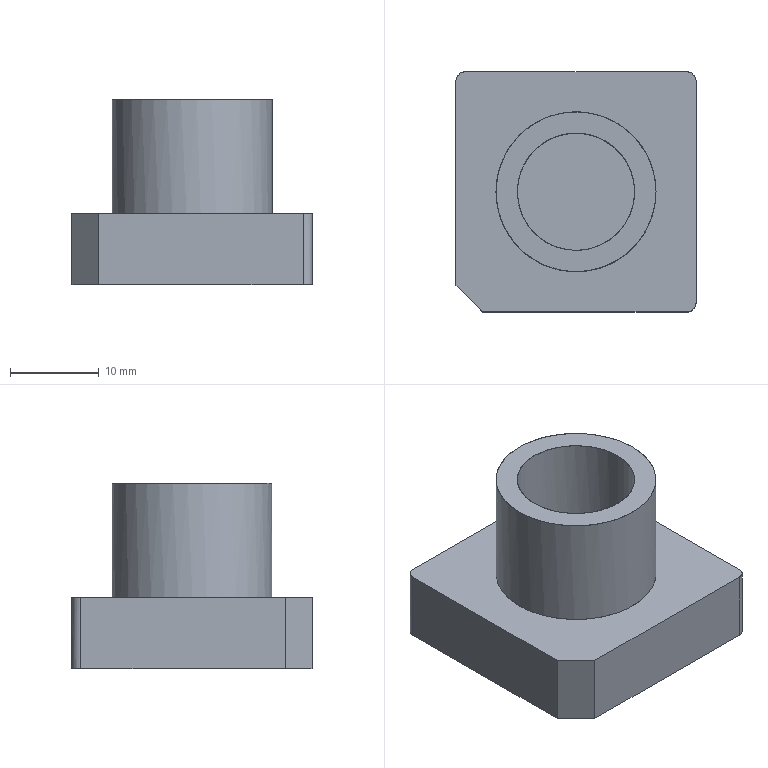NC program | PowerMill | posted with a generic post | part box 27 x 27 x 20.913 mm
Lines 4984 to 6006 of 92133:
N5081 M6
N5082 S18000 M03
N5083 G00 G90 X0.0 Y0.0
N5084 G43 Z9.8026 H2
N5085
N5086 G05 P10000 R4
N5087 X6.8917 Y9.7829
N5088 Z0.7935
N5089 G01 Z-0.4065 F3600.0
N5090 X6.8713 Y9.7747 F6000.0
N5091 G03 X6.762 Y9.5169 I0.0742 J-0.1836
N5092 G01 X7.2898 Y8.2119
N5093 X7.7468 Y7.8088
N5094 X8.2969 Y7.2124
N5095 X8.9814 Y6.3447
N5096 X9.6009 Y5.3686
N5097 X10.0822 Y4.3925
N5098 X10.451 Y3.4164
N5099 X10.7253 Y2.4403
N5100 X10.8209 Y1.9522
N5101 X10.9546 Y0.9761
N5102 X11.0 Y0.0
N5103 X10.9546 Y-0.9761
N5104 X10.8953 Y-1.4642
N5105 X10.7253 Y-2.4403
N5106 X10.451 Y-3.4164
N5107 X10.0822 Y-4.3925
N5108 X9.6009 Y-5.3686
N5109 X9.273 Y-5.9165
N5110 X8.6143 Y-6.8327
N5111 X7.8088 Y-7.7468
N5112 X7.2124 Y-8.2969
N5113 X6.3447 Y-8.9814
N5114 X5.3686 Y-9.6009
N5115 X4.3925 Y-10.0822
N5116 X3.4164 Y-10.4559
N5117 X2.3638 Y-10.7372
N5118 X1.9522 Y-10.8209
N5119 X0.9761 Y-10.9563
N5120 X0.0 Y-11.0
N5121 X-0.9761 Y-10.9546
N5122 X-1.9522 Y-10.8209
N5123 X-2.9283 Y-10.5992
N5124 X-3.9944 Y-10.2491
N5125 X-4.3925 Y-10.0822
N5126 X-5.3686 Y-9.6009
N5127 X-6.3447 Y-8.9814
N5128 X-7.222 Y-8.2969
N5129 X-7.7468 Y-7.8088
N5130 X-8.2041 Y-7.3208
N5131 X-8.6121 Y-6.8327
N5132 X-8.9814 Y-6.3447
N5133 X-9.6009 Y-5.3686
N5134 X-10.0822 Y-4.3925
N5135 X-10.451 Y-3.4164
N5136 X-10.5975 Y-2.9283
N5137 X-10.8241 Y-1.9522
N5138 X-10.9546 Y-0.9761
N5139 X-11.0 Y0.0
N5140 X-10.9546 Y0.9761
N5141 X-10.8241 Y1.9522
N5142 X-10.7198 Y2.4403
N5143 X-10.451 Y3.4164
N5144 X-10.0822 Y4.3925
N5145 X-9.6009 Y5.3686
N5146 X-9.3005 Y5.8566
N5147 X-8.7849 Y6.6104
N5148 X-8.2041 Y7.3208
N5149 X-7.8088 Y7.7468
N5150 X-7.222 Y8.2969
N5151 X-6.3447 Y8.9814
N5152 X-5.9008 Y9.273
N5153 X-5.0694 Y9.7611
N5154 X-3.9944 Y10.2491
N5155 X-2.9283 Y10.5992
N5156 X-1.9522 Y10.8209
N5157 X-0.9761 Y10.9546
N5158 X0.0 Y11.0
N5159 X0.9761 Y10.9563
N5160 X1.4642 Y10.8953
N5161 X2.3638 Y10.7372
N5162 X3.4164 Y10.4559
N5163 X4.3925 Y10.0822
N5164 X5.3686 Y9.6009
N5165 X6.3447 Y8.9814
N5166 X6.8327 Y8.6151
N5167 X7.2898 Y8.2119
N5168 X6.8917 Y9.7829 Z-0.606
N5169 X6.8713 Y9.7747
N5170 G03 X6.762 Y9.5169 I0.0742 J-0.1836
N5171 G01 X7.2898 Y8.2119
N5172 X7.7468 Y7.8088
N5173 X8.2969 Y7.2124
N5174 X8.9814 Y6.3447
N5175 X9.6009 Y5.3686
N5176 X10.0822 Y4.3925
N5177 X10.451 Y3.4164
N5178 X10.7253 Y2.4403
N5179 X10.8209 Y1.9522
N5180 X10.9546 Y0.9761
N5181 X11.0 Y0.0
N5182 X10.9546 Y-0.9761
N5183 X10.8953 Y-1.4642
N5184 X10.7253 Y-2.4403
N5185 X10.451 Y-3.4164
N5186 X10.0822 Y-4.3925
N5187 X9.6009 Y-5.3686
N5188 X9.273 Y-5.9165
N5189 X8.6143 Y-6.8327
N5190 X7.8088 Y-7.7468
N5191 X7.2124 Y-8.2969
N5192 X6.3447 Y-8.9814
N5193 X5.3686 Y-9.6009
N5194 X4.3925 Y-10.0822
N5195 X3.4164 Y-10.4559
N5196 X2.3638 Y-10.7372
N5197 X1.9522 Y-10.8209
N5198 X0.9761 Y-10.9563
N5199 X0.0 Y-11.0
N5200 X-0.9761 Y-10.9546
N5201 X-1.9522 Y-10.8209
N5202 X-2.9283 Y-10.5992
N5203 X-3.9944 Y-10.2491
N5204 X-4.3925 Y-10.0822
N5205 X-5.3686 Y-9.6009
N5206 X-6.3447 Y-8.9814
N5207 X-7.2221 Y-8.2969
N5208 X-7.7468 Y-7.8088
N5209 X-8.2041 Y-7.3208
N5210 X-8.6121 Y-6.8327
N5211 X-8.9814 Y-6.3447
N5212 X-9.6009 Y-5.3686
N5213 X-10.0822 Y-4.3925
N5214 X-10.451 Y-3.4164
N5215 X-10.5975 Y-2.9283
N5216 X-10.8241 Y-1.9522
N5217 X-10.9546 Y-0.9761
N5218 X-11.0 Y0.0
N5219 X-10.9546 Y0.9761
N5220 X-10.8241 Y1.9522
N5221 X-10.7198 Y2.4403
N5222 X-10.451 Y3.4164
N5223 X-10.0822 Y4.3925
N5224 X-9.6009 Y5.3686
N5225 X-9.3005 Y5.8566
N5226 X-8.7849 Y6.6104
N5227 X-8.2041 Y7.3208
N5228 X-7.8088 Y7.7468
N5229 X-7.2221 Y8.2969
N5230 X-6.3447 Y8.9814
N5231 X-5.9008 Y9.273
N5232 X-5.0694 Y9.7611
N5233 X-3.9944 Y10.2491
N5234 X-2.9283 Y10.5992
N5235 X-1.9522 Y10.8209
N5236 X-0.9761 Y10.9546
N5237 X0.0 Y11.0
N5238 X0.9761 Y10.9563
N5239 X1.4642 Y10.8953
N5240 X2.3638 Y10.7372
N5241 X3.4164 Y10.4559
N5242 X4.3925 Y10.0822
N5243 X5.3686 Y9.6009
N5244 X6.3447 Y8.9814
N5245 X6.8327 Y8.6151
N5246 X7.2898 Y8.2119
N5247 X6.8917 Y9.7829 Z-0.8056
N5248 X6.8713 Y9.7747
N5249 G03 X6.762 Y9.5169 I0.0742 J-0.1836
N5250 G01 X7.2898 Y8.2119
N5251 X7.7468 Y7.8088
N5252 X8.2969 Y7.2124
N5253 X8.9814 Y6.3447
N5254 X9.6009 Y5.3686
N5255 X10.0822 Y4.3925
N5256 X10.451 Y3.4164
N5257 X10.7253 Y2.4403
N5258 X10.8209 Y1.9522
N5259 X10.9546 Y0.9761
N5260 X11.0 Y0.0
N5261 X10.9546 Y-0.9761
N5262 X10.8953 Y-1.4642
N5263 X10.7253 Y-2.4403
N5264 X10.451 Y-3.4164
N5265 X10.0822 Y-4.3925
N5266 X9.6009 Y-5.3686
N5267 X9.273 Y-5.9165
N5268 X8.6143 Y-6.8327
N5269 X7.8088 Y-7.7468
N5270 X7.2124 Y-8.2969
N5271 X6.3447 Y-8.9814
N5272 X5.3686 Y-9.6009
N5273 X4.3925 Y-10.0822
N5274 X3.4164 Y-10.4559
N5275 X2.3638 Y-10.7372
N5276 X1.9522 Y-10.8209
N5277 X0.9761 Y-10.9563
N5278 X0.0 Y-11.0
N5279 X-0.9761 Y-10.9546
N5280 X-1.9522 Y-10.8209
N5281 X-2.9283 Y-10.5992
N5282 X-3.9944 Y-10.2491
N5283 X-4.3925 Y-10.0822
N5284 X-5.3686 Y-9.6009
N5285 X-6.3447 Y-8.9814
N5286 X-7.2221 Y-8.2969
N5287 X-7.7468 Y-7.8088
N5288 X-8.2041 Y-7.3208
N5289 X-8.6121 Y-6.8327
N5290 X-8.9814 Y-6.3447
N5291 X-9.6009 Y-5.3686
N5292 X-10.0822 Y-4.3925
N5293 X-10.451 Y-3.4164
N5294 X-10.5975 Y-2.9283
N5295 X-10.8241 Y-1.9522
N5296 X-10.9546 Y-0.9761
N5297 X-11.0 Y0.0
N5298 X-10.9546 Y0.9761
N5299 X-10.8241 Y1.9522
N5300 X-10.7198 Y2.4403
N5301 X-10.451 Y3.4164
N5302 X-10.0822 Y4.3925
N5303 X-9.6009 Y5.3686
N5304 X-9.3005 Y5.8566
N5305 X-8.7849 Y6.6104
N5306 X-8.2041 Y7.3208
N5307 X-7.8088 Y7.7468
N5308 X-7.2221 Y8.2969
N5309 X-6.3447 Y8.9814
N5310 X-5.9008 Y9.273
N5311 X-5.0694 Y9.7611
N5312 X-3.9944 Y10.2491
N5313 X-2.9283 Y10.5992
N5314 X-1.9522 Y10.8209
N5315 X-0.9761 Y10.9546
N5316 X0.0 Y11.0
N5317 X0.9761 Y10.9563
N5318 X1.4642 Y10.8953
N5319 X2.3638 Y10.7372
N5320 X3.4164 Y10.4559
N5321 X4.3925 Y10.0822
N5322 X5.3686 Y9.6009
N5323 X6.3447 Y8.9814
N5324 X6.8327 Y8.6151
N5325 X7.2898 Y8.2119
N5326 X6.8917 Y9.7829 Z-1.0051
N5327 X6.8713 Y9.7747
N5328 G03 X6.762 Y9.5169 I0.0742 J-0.1836
N5329 G01 X7.2898 Y8.2119
N5330 X7.7468 Y7.8088
N5331 X8.2969 Y7.2125
N5332 X8.9814 Y6.3447
N5333 X9.6009 Y5.3686
N5334 X10.0822 Y4.3925
N5335 X10.451 Y3.4164
N5336 X10.7253 Y2.4403
N5337 X10.8209 Y1.9522
N5338 X10.9546 Y0.9761
N5339 X11.0 Y0.0
N5340 X10.9546 Y-0.9761
N5341 X10.8953 Y-1.4642
N5342 X10.7253 Y-2.4403
N5343 X10.451 Y-3.4164
N5344 X10.0822 Y-4.3925
N5345 X9.6009 Y-5.3686
N5346 X9.273 Y-5.9165
N5347 X8.6143 Y-6.8327
N5348 X7.8088 Y-7.7468
N5349 X7.2125 Y-8.2969
N5350 X6.3447 Y-8.9814
N5351 X5.3686 Y-9.6009
N5352 X4.3925 Y-10.0822
N5353 X3.4164 Y-10.4559
N5354 X2.3638 Y-10.7372
N5355 X1.9522 Y-10.8209
N5356 X0.9761 Y-10.9563
N5357 X0.0 Y-11.0
N5358 X-0.9761 Y-10.9546
N5359 X-1.9522 Y-10.8209
N5360 X-2.9283 Y-10.5992
N5361 X-3.9944 Y-10.2491
N5362 X-4.3925 Y-10.0822
N5363 X-5.3686 Y-9.6009
N5364 X-6.3447 Y-8.9814
N5365 X-7.2221 Y-8.2969
N5366 X-7.7468 Y-7.8088
N5367 X-8.2041 Y-7.3208
N5368 X-8.6121 Y-6.8327
N5369 X-8.9814 Y-6.3447
N5370 X-9.6009 Y-5.3686
N5371 X-10.0822 Y-4.3925
N5372 X-10.451 Y-3.4164
N5373 X-10.5975 Y-2.9283
N5374 X-10.8241 Y-1.9522
N5375 X-10.9546 Y-0.9761
N5376 X-11.0 Y0.0
N5377 X-10.9546 Y0.9761
N5378 X-10.8241 Y1.9522
N5379 X-10.7198 Y2.4403
N5380 X-10.451 Y3.4164
N5381 X-10.0822 Y4.3925
N5382 X-9.6009 Y5.3686
N5383 X-9.3005 Y5.8566
N5384 X-8.7849 Y6.6104
N5385 X-8.2041 Y7.3208
N5386 X-7.8088 Y7.7468
N5387 X-7.2221 Y8.2969
N5388 X-6.3447 Y8.9814
N5389 X-5.9008 Y9.273
N5390 X-5.0694 Y9.7611
N5391 X-3.9944 Y10.2491
N5392 X-2.9283 Y10.5992
N5393 X-1.9522 Y10.8209
N5394 X-0.9761 Y10.9546
N5395 X0.0 Y11.0
N5396 X0.9761 Y10.9563
N5397 X1.4642 Y10.8953
N5398 X2.3638 Y10.7372
N5399 X3.4164 Y10.4559
N5400 X4.3925 Y10.0822
N5401 X5.3686 Y9.6009
N5402 X6.3447 Y8.9814
N5403 X6.8327 Y8.6151
N5404 X7.2898 Y8.2119
N5405 X6.8917 Y9.7829 Z-1.2046
N5406 X6.8713 Y9.7747
N5407 G03 X6.762 Y9.5169 I0.0742 J-0.1836
N5408 G01 X7.2898 Y8.212
N5409 X7.7468 Y7.8088
N5410 X8.2969 Y7.2125
N5411 X8.9814 Y6.3447
N5412 X9.6009 Y5.3686
N5413 X10.0822 Y4.3925
N5414 X10.451 Y3.4164
N5415 X10.7253 Y2.4403
N5416 X10.8209 Y1.9522
N5417 X10.9546 Y0.9761
N5418 X11.0 Y0.0
N5419 X10.9546 Y-0.9761
N5420 X10.8953 Y-1.4642
N5421 X10.7253 Y-2.4403
N5422 X10.451 Y-3.4164
N5423 X10.0822 Y-4.3925
N5424 X9.6009 Y-5.3686
N5425 X9.273 Y-5.9165
N5426 X8.6143 Y-6.8327
N5427 X7.8088 Y-7.7468
N5428 X7.2125 Y-8.2969
N5429 X6.3447 Y-8.9814
N5430 X5.3686 Y-9.6009
N5431 X4.3925 Y-10.0822
N5432 X3.4164 Y-10.4559
N5433 X2.3638 Y-10.7372
N5434 X1.9522 Y-10.8209
N5435 X0.9761 Y-10.9563
N5436 X0.0 Y-11.0
N5437 X-0.9761 Y-10.9546
N5438 X-1.9522 Y-10.8209
N5439 X-2.9283 Y-10.5992
N5440 X-3.9944 Y-10.2491
N5441 X-4.3925 Y-10.0822
N5442 X-5.3686 Y-9.6009
N5443 X-6.3447 Y-8.9814
N5444 X-7.2221 Y-8.2969
N5445 X-7.7468 Y-7.8088
N5446 X-8.2041 Y-7.3208
N5447 X-8.6121 Y-6.8327
N5448 X-8.9814 Y-6.3447
N5449 X-9.6009 Y-5.3686
N5450 X-10.0822 Y-4.3925
N5451 X-10.451 Y-3.4164
N5452 X-10.5975 Y-2.9283
N5453 X-10.8241 Y-1.9522
N5454 X-10.9546 Y-0.9761
N5455 X-11.0 Y0.0
N5456 X-10.9546 Y0.9761
N5457 X-10.8241 Y1.9522
N5458 X-10.7198 Y2.4403
N5459 X-10.451 Y3.4164
N5460 X-10.0822 Y4.3925
N5461 X-9.6009 Y5.3686
N5462 X-9.3005 Y5.8566
N5463 X-8.7849 Y6.6104
N5464 X-8.2041 Y7.3208
N5465 X-7.8088 Y7.7468
N5466 X-7.2221 Y8.2969
N5467 X-6.3447 Y8.9814
N5468 X-5.9008 Y9.273
N5469 X-5.0694 Y9.7611
N5470 X-3.9944 Y10.2491
N5471 X-2.9283 Y10.5992
N5472 X-1.9522 Y10.8209
N5473 X-0.9761 Y10.9546
N5474 X0.0 Y11.0
N5475 X0.9761 Y10.9563
N5476 X1.4642 Y10.8953
N5477 X2.3638 Y10.7372
N5478 X3.4164 Y10.4559
N5479 X4.3925 Y10.0822
N5480 X5.3686 Y9.6009
N5481 X6.3447 Y8.9814
N5482 X6.8327 Y8.6151
N5483 X7.2898 Y8.212
N5484 X6.8917 Y9.7829 Z-1.4041
N5485 X6.8713 Y9.7747
N5486 G03 X6.762 Y9.5169 I0.0742 J-0.1836
N5487 G01 X7.2898 Y8.212
N5488 X7.7468 Y7.8088
N5489 X8.2969 Y7.2125
N5490 X8.9814 Y6.3447
N5491 X9.6009 Y5.3686
N5492 X10.0822 Y4.3925
N5493 X10.451 Y3.4164
N5494 X10.7253 Y2.4403
N5495 X10.8209 Y1.9522
N5496 X10.9546 Y0.9761
N5497 X11.0 Y0.0
N5498 X10.9546 Y-0.9761
N5499 X10.8953 Y-1.4642
N5500 X10.7253 Y-2.4403
N5501 X10.451 Y-3.4164
N5502 X10.0822 Y-4.3925
N5503 X9.6009 Y-5.3686
N5504 X9.273 Y-5.9165
N5505 X8.6143 Y-6.8327
N5506 X7.8088 Y-7.7468
N5507 X7.2125 Y-8.2969
N5508 X6.3447 Y-8.9814
N5509 X5.3686 Y-9.6009
N5510 X4.3925 Y-10.0822
N5511 X3.4164 Y-10.4559
N5512 X2.3638 Y-10.7372
N5513 X1.9522 Y-10.8209
N5514 X0.9761 Y-10.9563
N5515 X0.0 Y-11.0
N5516 X-0.9761 Y-10.9546
N5517 X-1.9522 Y-10.8209
N5518 X-2.9283 Y-10.5992
N5519 X-3.9944 Y-10.2491
N5520 X-4.3925 Y-10.0822
N5521 X-5.3686 Y-9.6009
N5522 X-6.3447 Y-8.9814
N5523 X-7.2221 Y-8.2969
N5524 X-7.7468 Y-7.8088
N5525 X-8.2041 Y-7.3208
N5526 X-8.6121 Y-6.8327
N5527 X-8.9814 Y-6.3447
N5528 X-9.6009 Y-5.3686
N5529 X-10.0822 Y-4.3925
N5530 X-10.451 Y-3.4164
N5531 X-10.5975 Y-2.9283
N5532 X-10.8241 Y-1.9522
N5533 X-10.9546 Y-0.9761
N5534 X-11.0 Y0.0
N5535 X-10.9546 Y0.9761
N5536 X-10.8241 Y1.9522
N5537 X-10.7198 Y2.4403
N5538 X-10.451 Y3.4164
N5539 X-10.0822 Y4.3925
N5540 X-9.6009 Y5.3686
N5541 X-9.3005 Y5.8566
N5542 X-8.7849 Y6.6104
N5543 X-8.2041 Y7.3208
N5544 X-7.8088 Y7.7468
N5545 X-7.2221 Y8.2969
N5546 X-6.3447 Y8.9814
N5547 X-5.9008 Y9.273
N5548 X-5.0694 Y9.7611
N5549 X-3.9944 Y10.2491
N5550 X-2.9283 Y10.5992
N5551 X-1.9522 Y10.8209
N5552 X-0.9761 Y10.9546
N5553 X0.0 Y11.0
N5554 X0.9761 Y10.9563
N5555 X1.4642 Y10.8953
N5556 X2.3638 Y10.7372
N5557 X3.4164 Y10.4559
N5558 X4.3925 Y10.0822
N5559 X5.3686 Y9.6009
N5560 X6.3447 Y8.9814
N5561 X6.8327 Y8.6151
N5562 X7.2898 Y8.212
N5563 X6.8917 Y9.7829 Z-1.6037
N5564 X6.8713 Y9.7747
N5565 G03 X6.762 Y9.5169 I0.0742 J-0.1836
N5566 G01 X7.2898 Y8.212
N5567 X7.7468 Y7.8088
N5568 X8.2969 Y7.2125
N5569 X8.9814 Y6.3447
N5570 X9.6009 Y5.3686
N5571 X10.0822 Y4.3925
N5572 X10.451 Y3.4164
N5573 X10.7253 Y2.4403
N5574 X10.8209 Y1.9522
N5575 X10.9546 Y0.9761
N5576 X11.0 Y0.0
N5577 X10.9546 Y-0.9761
N5578 X10.8953 Y-1.4642
N5579 X10.7253 Y-2.4403
N5580 X10.451 Y-3.4164
N5581 X10.0822 Y-4.3925
N5582 X9.6009 Y-5.3686
N5583 X9.273 Y-5.9165
N5584 X8.6143 Y-6.8327
N5585 X7.8088 Y-7.7468
N5586 X7.2125 Y-8.2969
N5587 X6.3447 Y-8.9814
N5588 X5.3686 Y-9.6009
N5589 X4.3925 Y-10.0822
N5590 X3.4164 Y-10.4559
N5591 X2.3638 Y-10.7372
N5592 X1.9522 Y-10.8209
N5593 X0.9761 Y-10.9563
N5594 X0.0 Y-11.0
N5595 X-0.9761 Y-10.9546
N5596 X-1.9522 Y-10.8209
N5597 X-2.9283 Y-10.5992
N5598 X-3.9944 Y-10.2491
N5599 X-4.3925 Y-10.0822
N5600 X-5.3686 Y-9.6009
N5601 X-6.3447 Y-8.9814
N5602 X-7.2221 Y-8.2969
N5603 X-7.7468 Y-7.8088
N5604 X-8.2041 Y-7.3208
N5605 X-8.6121 Y-6.8327
N5606 X-8.9814 Y-6.3447
N5607 X-9.6009 Y-5.3686
N5608 X-10.0822 Y-4.3925
N5609 X-10.451 Y-3.4164
N5610 X-10.5975 Y-2.9283
N5611 X-10.8241 Y-1.9522
N5612 X-10.9546 Y-0.9761
N5613 X-11.0 Y0.0
N5614 X-10.9546 Y0.9761
N5615 X-10.8241 Y1.9522
N5616 X-10.7198 Y2.4403
N5617 X-10.451 Y3.4164
N5618 X-10.0822 Y4.3925
N5619 X-9.6009 Y5.3686
N5620 X-9.3005 Y5.8566
N5621 X-8.7849 Y6.6104
N5622 X-8.2041 Y7.3208
N5623 X-7.8088 Y7.7468
N5624 X-7.2221 Y8.2969
N5625 X-6.3447 Y8.9814
N5626 X-5.9008 Y9.273
N5627 X-5.0694 Y9.7611
N5628 X-3.9944 Y10.2491
N5629 X-2.9283 Y10.5992
N5630 X-1.9522 Y10.8209
N5631 X-0.9761 Y10.9546
N5632 X0.0 Y11.0
N5633 X0.9761 Y10.9563
N5634 X1.4642 Y10.8953
N5635 X2.3638 Y10.7372
N5636 X3.4164 Y10.4559
N5637 X4.3925 Y10.0822
N5638 X5.3686 Y9.6009
N5639 X6.3447 Y8.9814
N5640 X6.8327 Y8.6151
N5641 X7.2898 Y8.212
N5642 X6.8917 Y9.7829 Z-1.8032
N5643 X6.8713 Y9.7747
N5644 G03 X6.762 Y9.5169 I0.0742 J-0.1836
N5645 G01 X7.2898 Y8.212
N5646 X7.7468 Y7.8088
N5647 X8.2969 Y7.2125
N5648 X8.9814 Y6.3447
N5649 X9.6009 Y5.3686
N5650 X10.0822 Y4.3925
N5651 X10.451 Y3.4164
N5652 X10.7253 Y2.4403
N5653 X10.8209 Y1.9522
N5654 X10.9546 Y0.9761
N5655 X11.0 Y0.0
N5656 X10.9546 Y-0.9761
N5657 X10.8953 Y-1.4642
N5658 X10.7253 Y-2.4403
N5659 X10.451 Y-3.4164
N5660 X10.0822 Y-4.3925
N5661 X9.6009 Y-5.3686
N5662 X9.273 Y-5.9165
N5663 X8.6143 Y-6.8327
N5664 X7.8088 Y-7.7468
N5665 X7.2125 Y-8.2969
N5666 X6.3447 Y-8.9814
N5667 X5.3686 Y-9.6009
N5668 X4.3925 Y-10.0822
N5669 X3.4164 Y-10.4559
N5670 X2.3638 Y-10.7372
N5671 X1.9522 Y-10.8209
N5672 X0.9761 Y-10.9563
N5673 X0.0 Y-11.0
N5674 X-0.9761 Y-10.9546
N5675 X-1.9522 Y-10.8209
N5676 X-2.9283 Y-10.5992
N5677 X-3.9944 Y-10.2491
N5678 X-4.3925 Y-10.0822
N5679 X-5.3686 Y-9.6009
N5680 X-6.3447 Y-8.9814
N5681 X-7.2221 Y-8.2969
N5682 X-7.7468 Y-7.8088
N5683 X-8.2041 Y-7.3208
N5684 X-8.6121 Y-6.8327
N5685 X-8.9814 Y-6.3447
N5686 X-9.6009 Y-5.3686
N5687 X-10.0822 Y-4.3925
N5688 X-10.451 Y-3.4164
N5689 X-10.5975 Y-2.9283
N5690 X-10.8241 Y-1.9522
N5691 X-10.9546 Y-0.9761
N5692 X-11.0 Y0.0
N5693 X-10.9546 Y0.9761
N5694 X-10.8241 Y1.9522
N5695 X-10.7198 Y2.4403
N5696 X-10.451 Y3.4164
N5697 X-10.0822 Y4.3925
N5698 X-9.6009 Y5.3686
N5699 X-9.3005 Y5.8566
N5700 X-8.7849 Y6.6104
N5701 X-8.2041 Y7.3208
N5702 X-7.8088 Y7.7468
N5703 X-7.2221 Y8.2969
N5704 X-6.3447 Y8.9814
N5705 X-5.9008 Y9.273
N5706 X-5.0694 Y9.7611
N5707 X-3.9944 Y10.2491
N5708 X-2.9283 Y10.5992
N5709 X-1.9522 Y10.8209
N5710 X-0.9761 Y10.9546
N5711 X0.0 Y11.0
N5712 X0.9761 Y10.9563
N5713 X1.4642 Y10.8953
N5714 X2.3638 Y10.7372
N5715 X3.4164 Y10.4559
N5716 X4.3925 Y10.0822
N5717 X5.3686 Y9.6009
N5718 X6.3447 Y8.9814
N5719 X6.8327 Y8.6151
N5720 X7.2898 Y8.212
N5721 X6.8917 Y9.7829 Z-2.0027
N5722 X6.8713 Y9.7747
N5723 G03 X6.762 Y9.5169 I0.0742 J-0.1836
N5724 G01 X7.2898 Y8.212
N5725 X7.7468 Y7.8088
N5726 X8.2969 Y7.2125
N5727 X8.9814 Y6.3447
N5728 X9.6009 Y5.3686
N5729 X10.0822 Y4.3925
N5730 X10.451 Y3.4164
N5731 X10.7253 Y2.4403
N5732 X10.8209 Y1.9522
N5733 X10.9546 Y0.9761
N5734 X11.0 Y0.0
N5735 X10.9546 Y-0.9761
N5736 X10.8953 Y-1.4642
N5737 X10.7253 Y-2.4403
N5738 X10.451 Y-3.4164
N5739 X10.0822 Y-4.3925
N5740 X9.6009 Y-5.3686
N5741 X9.273 Y-5.9165
N5742 X8.6143 Y-6.8327
N5743 X7.8088 Y-7.7468
N5744 X7.2125 Y-8.2969
N5745 X6.3447 Y-8.9814
N5746 X5.3686 Y-9.6009
N5747 X4.3925 Y-10.0822
N5748 X3.4164 Y-10.4559
N5749 X2.3638 Y-10.7372
N5750 X1.9522 Y-10.8209
N5751 X0.9761 Y-10.9563
N5752 X0.0 Y-11.0
N5753 X-0.9761 Y-10.9546
N5754 X-1.9522 Y-10.8209
N5755 X-2.9283 Y-10.5992
N5756 X-3.9944 Y-10.2491
N5757 X-4.3925 Y-10.0822
N5758 X-5.3686 Y-9.6009
N5759 X-6.3447 Y-8.9814
N5760 X-7.2221 Y-8.2969
N5761 X-7.7468 Y-7.8088
N5762 X-8.2041 Y-7.3208
N5763 X-8.6122 Y-6.8327
N5764 X-8.9814 Y-6.3447
N5765 X-9.6009 Y-5.3686
N5766 X-10.0822 Y-4.3925
N5767 X-10.451 Y-3.4164
N5768 X-10.5975 Y-2.9283
N5769 X-10.8241 Y-1.9522
N5770 X-10.9546 Y-0.9761
N5771 X-11.0 Y0.0
N5772 X-10.9546 Y0.9761
N5773 X-10.8241 Y1.9522
N5774 X-10.7198 Y2.4403
N5775 X-10.451 Y3.4164
N5776 X-10.0822 Y4.3925
N5777 X-9.6009 Y5.3686
N5778 X-9.3005 Y5.8566
N5779 X-8.7849 Y6.6104
N5780 X-8.2041 Y7.3208
N5781 X-7.8088 Y7.7468
N5782 X-7.2221 Y8.2969
N5783 X-6.3447 Y8.9814
N5784 X-5.9008 Y9.273
N5785 X-5.0694 Y9.7611
N5786 X-3.9944 Y10.2491
N5787 X-2.9283 Y10.5992
N5788 X-1.9522 Y10.8209
N5789 X-0.9761 Y10.9546
N5790 X0.0 Y11.0
N5791 X0.9761 Y10.9563
N5792 X1.4642 Y10.8953
N5793 X2.3638 Y10.7372
N5794 X3.4164 Y10.4559
N5795 X4.3925 Y10.0822
N5796 X5.3686 Y9.6009
N5797 X6.3447 Y8.9814
N5798 X6.8327 Y8.6151
N5799 X7.2898 Y8.212
N5800 X6.8917 Y9.7829 Z-2.2022
N5801 X6.8713 Y9.7747
N5802 G03 X6.762 Y9.5169 I0.0742 J-0.1836
N5803 G01 X7.2898 Y8.212
N5804 X7.7468 Y7.8088
N5805 X8.2969 Y7.2125
N5806 X8.9814 Y6.3447
N5807 X9.6009 Y5.3686
N5808 X10.0822 Y4.3925
N5809 X10.451 Y3.4164
N5810 X10.7253 Y2.4403
N5811 X10.8209 Y1.9522
N5812 X10.9546 Y0.9761
N5813 X11.0 Y0.0
N5814 X10.9546 Y-0.9761
N5815 X10.8953 Y-1.4642
N5816 X10.7253 Y-2.4403
N5817 X10.451 Y-3.4164
N5818 X10.0822 Y-4.3925
N5819 X9.6009 Y-5.3686
N5820 X9.273 Y-5.9165
N5821 X8.6143 Y-6.8327
N5822 X7.8088 Y-7.7468
N5823 X7.2125 Y-8.2969
N5824 X6.3447 Y-8.9814
N5825 X5.3686 Y-9.6009
N5826 X4.3925 Y-10.0822
N5827 X3.4164 Y-10.4559
N5828 X2.3638 Y-10.7372
N5829 X1.9522 Y-10.8209
N5830 X0.9761 Y-10.9563
N5831 X0.0 Y-11.0
N5832 X-0.9761 Y-10.9546
N5833 X-1.9522 Y-10.8209
N5834 X-2.9283 Y-10.5992
N5835 X-3.9944 Y-10.2491
N5836 X-4.3925 Y-10.0822
N5837 X-5.3686 Y-9.6009
N5838 X-6.3447 Y-8.9814
N5839 X-7.2221 Y-8.2969
N5840 X-7.7468 Y-7.8088
N5841 X-8.2041 Y-7.3208
N5842 X-8.6122 Y-6.8327
N5843 X-8.9814 Y-6.3447
N5844 X-9.6009 Y-5.3686
N5845 X-10.0822 Y-4.3925
N5846 X-10.451 Y-3.4164
N5847 X-10.5975 Y-2.9283
N5848 X-10.8241 Y-1.9522
N5849 X-10.9546 Y-0.9761
N5850 X-11.0 Y0.0
N5851 X-10.9546 Y0.9761
N5852 X-10.8241 Y1.9522
N5853 X-10.7198 Y2.4403
N5854 X-10.451 Y3.4164
N5855 X-10.0822 Y4.3925
N5856 X-9.6009 Y5.3686
N5857 X-9.3005 Y5.8566
N5858 X-8.7849 Y6.6104
N5859 X-8.2041 Y7.3208
N5860 X-7.8088 Y7.7468
N5861 X-7.2221 Y8.2969
N5862 X-6.3447 Y8.9814
N5863 X-5.9008 Y9.273
N5864 X-5.0694 Y9.7611
N5865 X-3.9944 Y10.2491
N5866 X-2.9283 Y10.5992
N5867 X-1.9522 Y10.8209
N5868 X-0.9761 Y10.9546
N5869 X0.0 Y11.0
N5870 X0.9761 Y10.9563
N5871 X1.4642 Y10.8953
N5872 X2.3638 Y10.7372
N5873 X3.4164 Y10.4559
N5874 X4.3925 Y10.0822
N5875 X5.3686 Y9.6009
N5876 X6.3447 Y8.9814
N5877 X6.8327 Y8.6151
N5878 X7.2898 Y8.212
N5879 X6.8917 Y9.7829 Z-2.4018
N5880 X6.8713 Y9.7747
N5881 G03 X6.762 Y9.5169 I0.0742 J-0.1836
N5882 G01 X7.2898 Y8.212
N5883 X7.7468 Y7.8088
N5884 X8.2969 Y7.2125
N5885 X8.9814 Y6.3447
N5886 X9.6009 Y5.3686
N5887 X10.0822 Y4.3925
N5888 X10.451 Y3.4164
N5889 X10.7253 Y2.4403
N5890 X10.8209 Y1.9522
N5891 X10.9546 Y0.9761
N5892 X11.0 Y0.0
N5893 X10.9546 Y-0.9761
N5894 X10.8953 Y-1.4642
N5895 X10.7253 Y-2.4403
N5896 X10.451 Y-3.4164
N5897 X10.0822 Y-4.3925
N5898 X9.6009 Y-5.3686
N5899 X9.273 Y-5.9165
N5900 X8.6143 Y-6.8327
N5901 X7.8088 Y-7.7468
N5902 X7.2125 Y-8.2969
N5903 X6.3447 Y-8.9814
N5904 X5.3686 Y-9.6009
N5905 X4.3925 Y-10.0822
N5906 X3.4164 Y-10.4559
N5907 X2.3638 Y-10.7372
N5908 X1.9522 Y-10.8209
N5909 X0.9761 Y-10.9563
N5910 X0.0 Y-11.0
N5911 X-0.9761 Y-10.9546
N5912 X-1.9522 Y-10.8209
N5913 X-2.9283 Y-10.5992
N5914 X-3.9944 Y-10.2491
N5915 X-4.3925 Y-10.0822
N5916 X-5.3686 Y-9.6009
N5917 X-6.3447 Y-8.9814
N5918 X-7.2221 Y-8.2969
N5919 X-7.7468 Y-7.8088
N5920 X-8.2041 Y-7.3208
N5921 X-8.6122 Y-6.8327
N5922 X-8.9814 Y-6.3447
N5923 X-9.6009 Y-5.3686
N5924 X-10.0822 Y-4.3925
N5925 X-10.451 Y-3.4164
N5926 X-10.5975 Y-2.9283
N5927 X-10.8241 Y-1.9522
N5928 X-10.9546 Y-0.9761
N5929 X-11.0 Y0.0
N5930 X-10.9546 Y0.9761
N5931 X-10.8241 Y1.9522
N5932 X-10.7198 Y2.4403
N5933 X-10.451 Y3.4164
N5934 X-10.0822 Y4.3925
N5935 X-9.6009 Y5.3686
N5936 X-9.3005 Y5.8566
N5937 X-8.7849 Y6.6104
N5938 X-8.2041 Y7.3208
N5939 X-7.8088 Y7.7468
N5940 X-7.2221 Y8.2969
N5941 X-6.3447 Y8.9814
N5942 X-5.9008 Y9.273
N5943 X-5.0694 Y9.7611
N5944 X-3.9944 Y10.2491
N5945 X-2.9283 Y10.5992
N5946 X-1.9522 Y10.8209
N5947 X-0.9761 Y10.9546
N5948 X0.0 Y11.0
N5949 X0.9761 Y10.9563
N5950 X1.4642 Y10.8953
N5951 X2.3638 Y10.7372
N5952 X3.4164 Y10.4559
N5953 X4.3925 Y10.0822
N5954 X5.3686 Y9.6009
N5955 X6.3447 Y8.9814
N5956 X6.8327 Y8.6151
N5957 X7.2898 Y8.212
N5958 X6.8917 Y9.7829 Z-2.6013
N5959 X6.8713 Y9.7747
N5960 G03 X6.762 Y9.5169 I0.0742 J-0.1836
N5961 G01 X7.2898 Y8.212
N5962 X7.7468 Y7.8088
N5963 X8.2969 Y7.2125
N5964 X8.9814 Y6.3447
N5965 X9.6009 Y5.3686
N5966 X10.0822 Y4.3925
N5967 X10.451 Y3.4164
N5968 X10.7253 Y2.4403
N5969 X10.821 Y1.9522
N5970 X10.9547 Y0.9761
N5971 X11.0 Y0.0
N5972 X10.9547 Y-0.9761
N5973 X10.8953 Y-1.4642
N5974 X10.7253 Y-2.4403
N5975 X10.451 Y-3.4164
N5976 X10.0822 Y-4.3925
N5977 X9.6009 Y-5.3686
N5978 X9.273 Y-5.9165
N5979 X8.6143 Y-6.8327
N5980 X7.8088 Y-7.7468
N5981 X7.2125 Y-8.2969
N5982 X6.3447 Y-8.9814
N5983 X5.3686 Y-9.6009
N5984 X4.3925 Y-10.0822
N5985 X3.4164 Y-10.4559
N5986 X2.3638 Y-10.7372
N5987 X1.9522 Y-10.821
N5988 X0.9761 Y-10.9563
N5989 X0.0 Y-11.0
N5990 X-0.9761 Y-10.9547
N5991 X-1.9522 Y-10.821
N5992 X-2.9283 Y-10.5992
N5993 X-3.9944 Y-10.2491
N5994 X-4.3925 Y-10.0822
N5995 X-5.3686 Y-9.6009
N5996 X-6.3447 Y-8.9814
N5997 X-7.2221 Y-8.2969
N5998 X-7.7468 Y-7.8088
N5999 X-8.2042 Y-7.3208
N6000 X-8.6122 Y-6.8327
N6001 X-8.9814 Y-6.3447
N6002 X-9.6009 Y-5.3686
N6003 X-10.0822 Y-4.3925
N6004 X-10.451 Y-3.4164
N6005 X-10.5975 Y-2.9283
N6006 X-10.8241 Y-1.9522
N6007 X-10.9547 Y-0.9761
N6008 X-11.0 Y0.0
N6009 X-10.9547 Y0.9761
N6010 X-10.8241 Y1.9522
N6011 X-10.7198 Y2.4403
N6012 X-10.451 Y3.4164
N6013 X-10.0822 Y4.3925
N6014 X-9.6009 Y5.3686
N6015 X-9.3005 Y5.8566
N6016 X-8.7849 Y6.6104
N6017 X-8.2042 Y7.3208
N6018 X-7.8088 Y7.7468
N6019 X-7.2221 Y8.2969
N6020 X-6.3447 Y8.9814
N6021 X-5.9008 Y9.273
N6022 X-5.0694 Y9.7611
N6023 X-3.9944 Y10.2491
N6024 X-2.9283 Y10.5992
N6025 X-1.9522 Y10.821
N6026 X-0.9761 Y10.9547
N6027 X0.0 Y11.0
N6028 X0.9761 Y10.9563
N6029 X1.4642 Y10.8953
N6030 X2.3638 Y10.7372
N6031 X3.4164 Y10.4559
N6032 X4.3925 Y10.0822
N6033 X5.3686 Y9.6009
N6034 X6.3447 Y8.9814
N6035 X6.8327 Y8.6151
N6036 X7.2898 Y8.212
N6037 X6.8917 Y9.7829 Z-2.8008
N6038 X6.8713 Y9.7747
N6039 G03 X6.762 Y9.5169 I0.0742 J-0.1836
N6040 G01 X7.2898 Y8.212
N6041 X7.7468 Y7.8088
N6042 X8.2969 Y7.2125
N6043 X8.9814 Y6.3447
N6044 X9.6009 Y5.3686
N6045 X10.0822 Y4.3925
N6046 X10.451 Y3.4164
N6047 X10.7253 Y2.4403
N6048 X10.821 Y1.9522
N6049 X10.9547 Y0.9761
N6050 X11.0 Y0.0
N6051 X10.9547 Y-0.9761
N6052 X10.8953 Y-1.4642
N6053 X10.7253 Y-2.4403
N6054 X10.451 Y-3.4164
N6055 X10.0822 Y-4.3925
N6056 X9.6009 Y-5.3686
N6057 X9.273 Y-5.9165
N6058 X8.6143 Y-6.8327
N6059 X7.8088 Y-7.7468
N6060 X7.2125 Y-8.2969
N6061 X6.3447 Y-8.9814
N6062 X5.3686 Y-9.6009
N6063 X4.3925 Y-10.0822
N6064 X3.4164 Y-10.4559
N6065 X2.3638 Y-10.7372
N6066 X1.9522 Y-10.821
N6067 X0.9761 Y-10.9563
N6068 X0.0 Y-11.0
N6069 X-0.9761 Y-10.9547
N6070 X-1.9522 Y-10.821
N6071 X-2.9283 Y-10.5992
N6072 X-3.9944 Y-10.2491
N6073 X-4.3925 Y-10.0822
N6074 X-5.3686 Y-9.6009
N6075 X-6.3447 Y-8.9814
N6076 X-7.2221 Y-8.2969
N6077 X-7.7468 Y-7.8088
N6078 X-8.2042 Y-7.3208
N6079 X-8.6122 Y-6.8327
N6080 X-8.9814 Y-6.3447
N6081 X-9.6009 Y-5.3686
N6082 X-10.0822 Y-4.3925
N6083 X-10.451 Y-3.4164
N6084 X-10.5975 Y-2.9283
N6085 X-10.8241 Y-1.9522
N6086 X-10.9547 Y-0.9761
N6087 X-11.0 Y0.0
N6088 X-10.9547 Y0.9761
N6089 X-10.8241 Y1.9522
N6090 X-10.7198 Y2.4403
N6091 X-10.451 Y3.4164
N6092 X-10.0822 Y4.3925
N6093 X-9.6009 Y5.3686
N6094 X-9.3005 Y5.8566
N6095 X-8.7849 Y6.6104
N6096 X-8.2042 Y7.3208
N6097 X-7.8088 Y7.7468
N6098 X-7.2221 Y8.2969
N6099 X-6.3447 Y8.9814
N6100 X-5.9008 Y9.273
N6101 X-5.0694 Y9.7611
N6102 X-3.9944 Y10.2491
N6103 X-2.9283 Y10.5992